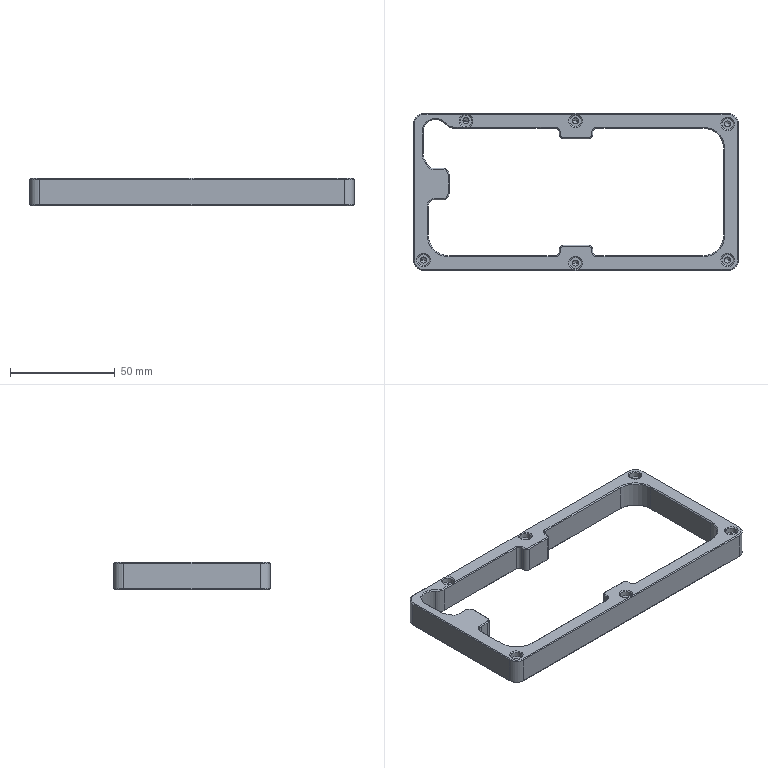Part | SolidWorks | features Chamfer 2, Extrusion 1, HoleWzd 1 | 1 solid | 186 faces | box 155.3 x 75 x 13.1 mm | volume 42362 mm3 | cone 71 | plane 68 | cylinder 47 | commonest cylinder face diameters 2.9 x12 5.5 x12 4 x8 10 x6 6 x4 20 x3